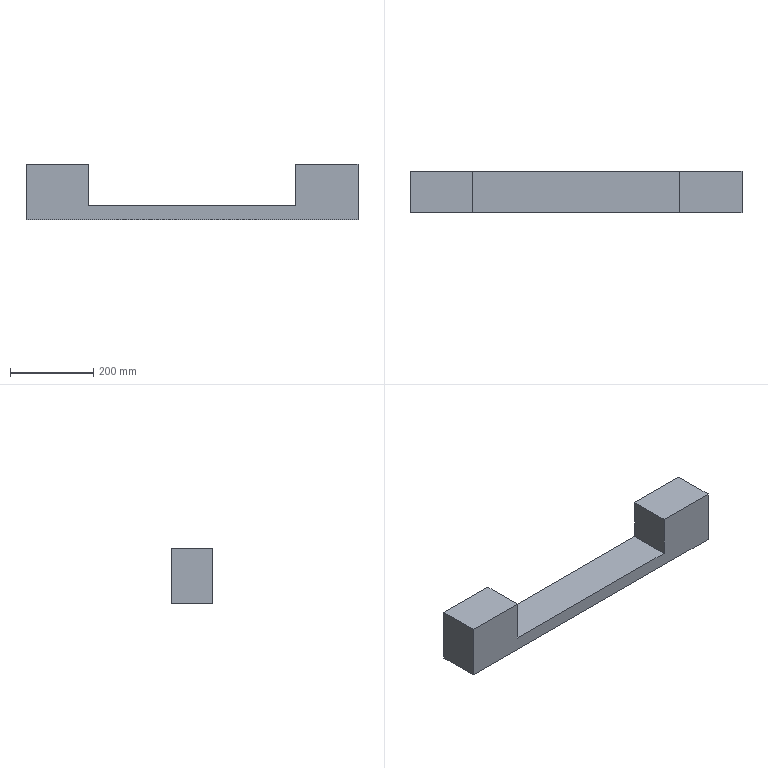Part | SolidWorks | features Split 3, Cut 2, Extrusion 1, MirrorPattern 1 | 1 solid | 20 faces | box 800 x 100 x 134 mm | volume 4312000 mm3 | plane 20
STEP:
#1=CARTESIAN_POINT('',(250.,100.,-33.));
#2=VERTEX_POINT('',#1);
#3=CARTESIAN_POINT('',(-250.,100.,-33.));
#4=VERTEX_POINT('',#3);
#5=CARTESIAN_POINT('',(-250.,100.,-33.));
#6=DIRECTION('',(-1.,0.,0.));
#7=VECTOR('',#6,1000.);
#8=LINE('',#5,#7);
#9=EDGE_CURVE('',#2,#4,#8,.T.);
#10=ORIENTED_EDGE('',*,*,#9,.F.);
#11=CARTESIAN_POINT('',(250.,100.,67.));
#12=VERTEX_POINT('',#11);
#13=CARTESIAN_POINT('',(250.,100.,167.));
#14=DIRECTION('',(0.,0.,-1.));
#15=VECTOR('',#14,1000.);
#16=LINE('',#13,#15);
#17=EDGE_CURVE('',#12,#2,#16,.T.);
#18=ORIENTED_EDGE('',*,*,#17,.F.);
#19=CARTESIAN_POINT('',(400.,100.,67.));
#20=VERTEX_POINT('',#19);
#21=CARTESIAN_POINT('',(-400.,100.,67.));
#22=DIRECTION('',(1.,0.,0.));
#23=VECTOR('',#22,1000.);
#24=LINE('',#21,#23);
#25=EDGE_CURVE('',#12,#20,#24,.T.);
#26=ORIENTED_EDGE('',*,*,#25,.T.);
#27=CARTESIAN_POINT('',(400.,100.,-67.));
#28=VERTEX_POINT('',#27);
#29=CARTESIAN_POINT('',(400.,100.,67.));
#30=DIRECTION('',(0.,0.,-1.));
#31=VECTOR('',#30,1000.);
#32=LINE('',#29,#31);
#33=EDGE_CURVE('',#20,#28,#32,.T.);
#34=ORIENTED_EDGE('',*,*,#33,.T.);
#35=CARTESIAN_POINT('',(-400.,100.,-67.));
#36=VERTEX_POINT('',#35);
#37=CARTESIAN_POINT('',(-400.,100.,-67.));
#38=DIRECTION('',(-1.,0.,0.));
#39=VECTOR('',#38,1000.);
#40=LINE('',#37,#39);
#41=EDGE_CURVE('',#28,#36,#40,.T.);
#42=ORIENTED_EDGE('',*,*,#41,.T.);
#43=CARTESIAN_POINT('',(-400.,100.,67.));
#44=VERTEX_POINT('',#43);
#45=CARTESIAN_POINT('',(-400.,100.,67.));
#46=DIRECTION('',(0.,0.,1.));
#47=VECTOR('',#46,1000.);
#48=LINE('',#45,#47);
#49=EDGE_CURVE('',#36,#44,#48,.T.);
#50=ORIENTED_EDGE('',*,*,#49,.T.);
#51=CARTESIAN_POINT('',(-250.,100.,67.));
#52=VERTEX_POINT('',#51);
#53=CARTESIAN_POINT('',(-400.,100.,67.));
#54=DIRECTION('',(1.,0.,0.));
#55=VECTOR('',#54,1000.);
#56=LINE('',#53,#55);
#57=EDGE_CURVE('',#44,#52,#56,.T.);
#58=ORIENTED_EDGE('',*,*,#57,.T.);
#59=CARTESIAN_POINT('',(-250.,100.,167.));
#60=DIRECTION('',(0.,0.,1.));
#61=VECTOR('',#60,1000.);
#62=LINE('',#59,#61);
#63=EDGE_CURVE('',#4,#52,#62,.T.);
#64=ORIENTED_EDGE('',*,*,#63,.F.);
#65=EDGE_LOOP('',(#10,#18,#26,#34,#42,#50,#58,#64));
#66=FACE_OUTER_BOUND('',#65,.T.);
#67=CARTESIAN_POINT('',(-380.,100.,47.));
#68=VERTEX_POINT('',#67);
#69=CARTESIAN_POINT('',(-270.,100.,47.));
#70=VERTEX_POINT('',#69);
#71=CARTESIAN_POINT('',(-380.,100.,47.));
#72=DIRECTION('',(1.,0.,0.));
#73=VECTOR('',#72,1000.);
#74=LINE('',#71,#73);
#75=EDGE_CURVE('',#68,#70,#74,.T.);
#76=ORIENTED_EDGE('',*,*,#75,.F.);
#77=CARTESIAN_POINT('',(-380.,100.,-33.));
#78=VERTEX_POINT('',#77);
#79=CARTESIAN_POINT('',(-380.,100.,47.));
#80=DIRECTION('',(0.,0.,1.));
#81=VECTOR('',#80,1000.);
#82=LINE('',#79,#81);
#83=EDGE_CURVE('',#78,#68,#82,.T.);
#84=ORIENTED_EDGE('',*,*,#83,.F.);
#85=CARTESIAN_POINT('',(-270.,100.,-33.));
#86=VERTEX_POINT('',#85);
#87=CARTESIAN_POINT('',(-380.,100.,-33.));
#88=DIRECTION('',(-1.,0.,0.));
#89=VECTOR('',#88,1000.);
#90=LINE('',#87,#89);
#91=EDGE_CURVE('',#86,#78,#90,.T.);
#92=ORIENTED_EDGE('',*,*,#91,.F.);
#93=CARTESIAN_POINT('',(-270.,100.,47.));
#94=DIRECTION('',(0.,0.,-1.));
#95=VECTOR('',#94,1000.);
#96=LINE('',#93,#95);
#97=EDGE_CURVE('',#70,#86,#96,.T.);
#98=ORIENTED_EDGE('',*,*,#97,.F.);
#99=EDGE_LOOP('',(#76,#84,#92,#98));
#100=FACE_BOUND('',#99,.T.);
#101=CARTESIAN_POINT('',(380.,100.,-33.));
#102=VERTEX_POINT('',#101);
#103=CARTESIAN_POINT('',(380.,100.,47.));
#104=VERTEX_POINT('',#103);
#105=CARTESIAN_POINT('',(380.,100.,47.));
#106=DIRECTION('',(0.,0.,1.));
#107=VECTOR('',#106,1000.);
#108=LINE('',#105,#107);
#109=EDGE_CURVE('',#102,#104,#108,.T.);
#110=ORIENTED_EDGE('',*,*,#109,.T.);
#111=CARTESIAN_POINT('',(270.,100.,47.));
#112=VERTEX_POINT('',#111);
#113=CARTESIAN_POINT('',(380.,100.,47.));
#114=DIRECTION('',(-1.,0.,0.));
#115=VECTOR('',#114,1000.);
#116=LINE('',#113,#115);
#117=EDGE_CURVE('',#104,#112,#116,.T.);
#118=ORIENTED_EDGE('',*,*,#117,.T.);
#119=CARTESIAN_POINT('',(270.,100.,-33.));
#120=VERTEX_POINT('',#119);
#121=CARTESIAN_POINT('',(270.,100.,47.));
#122=DIRECTION('',(0.,0.,-1.));
#123=VECTOR('',#122,1000.);
#124=LINE('',#121,#123);
#125=EDGE_CURVE('',#112,#120,#124,.T.);
#126=ORIENTED_EDGE('',*,*,#125,.T.);
#127=CARTESIAN_POINT('',(380.,100.,-33.));
#128=DIRECTION('',(1.,0.,0.));
#129=VECTOR('',#128,1000.);
#130=LINE('',#127,#129);
#131=EDGE_CURVE('',#120,#102,#130,.T.);
#132=ORIENTED_EDGE('',*,*,#131,.T.);
#133=EDGE_LOOP('',(#110,#118,#126,#132));
#134=FACE_BOUND('',#133,.T.);
#135=CARTESIAN_POINT('',(0.,100.,0.));
#136=DIRECTION('',(0.,-1.,0.));
#137=DIRECTION('',(0.,0.,-1.));
#138=AXIS2_PLACEMENT_3D('',#135,#136,#137);
#139=PLANE('',#138);
#140=ADVANCED_FACE('',(#66,#100,#134),#139,.F.);
#141=ORIENTED_EDGE('',*,*,#25,.F.);
#142=CARTESIAN_POINT('',(250.,0.,67.));
#143=VERTEX_POINT('',#142);
#144=CARTESIAN_POINT('',(250.,100.,67.));
#145=DIRECTION('',(0.,-1.,0.));
#146=VECTOR('',#145,1000.);
#147=LINE('',#144,#146);
#148=EDGE_CURVE('',#12,#143,#147,.T.);
#149=ORIENTED_EDGE('',*,*,#148,.T.);
#150=CARTESIAN_POINT('',(400.,0.,67.));
#151=VERTEX_POINT('',#150);
#152=CARTESIAN_POINT('',(-400.,0.,67.));
#153=DIRECTION('',(1.,0.,0.));
#154=VECTOR('',#153,1000.);
#155=LINE('',#152,#154);
#156=EDGE_CURVE('',#143,#151,#155,.T.);
#157=ORIENTED_EDGE('',*,*,#156,.T.);
#158=CARTESIAN_POINT('',(400.,100.,67.));
#159=DIRECTION('',(0.,-1.,0.));
#160=VECTOR('',#159,1000.);
#161=LINE('',#158,#160);
#162=EDGE_CURVE('',#20,#151,#161,.T.);
#163=ORIENTED_EDGE('',*,*,#162,.F.);
#164=EDGE_LOOP('',(#141,#149,#157,#163));
#165=FACE_OUTER_BOUND('',#164,.T.);
#166=CARTESIAN_POINT('',(-400.,100.,67.));
#167=DIRECTION('',(0.,0.,-1.));
#168=DIRECTION('',(-1.,0.,0.));
#169=AXIS2_PLACEMENT_3D('',#166,#167,#168);
#170=PLANE('',#169);
#171=ADVANCED_FACE('',(#165),#170,.F.);
#172=CARTESIAN_POINT('',(400.,0.,-67.));
#173=VERTEX_POINT('',#172);
#174=CARTESIAN_POINT('',(400.,0.,67.));
#175=DIRECTION('',(0.,0.,-1.));
#176=VECTOR('',#175,1000.);
#177=LINE('',#174,#176);
#178=EDGE_CURVE('',#151,#173,#177,.T.);
#179=ORIENTED_EDGE('',*,*,#178,.T.);
#180=CARTESIAN_POINT('',(400.,100.,-67.));
#181=DIRECTION('',(0.,-1.,0.));
#182=VECTOR('',#181,1000.);
#183=LINE('',#180,#182);
#184=EDGE_CURVE('',#28,#173,#183,.T.);
#185=ORIENTED_EDGE('',*,*,#184,.F.);
#186=ORIENTED_EDGE('',*,*,#33,.F.);
#187=ORIENTED_EDGE('',*,*,#162,.T.);
#188=EDGE_LOOP('',(#179,#185,#186,#187));
#189=FACE_OUTER_BOUND('',#188,.T.);
#190=CARTESIAN_POINT('',(400.,100.,67.));
#191=DIRECTION('',(-1.,0.,0.));
#192=DIRECTION('',(0.,0.,1.));
#193=AXIS2_PLACEMENT_3D('',#190,#191,#192);
#194=PLANE('',#193);
#195=ADVANCED_FACE('',(#189),#194,.F.);
#196=CARTESIAN_POINT('',(-400.,0.,-67.));
#197=VERTEX_POINT('',#196);
#198=CARTESIAN_POINT('',(-400.,0.,-67.));
#199=DIRECTION('',(-1.,0.,0.));
#200=VECTOR('',#199,1000.);
#201=LINE('',#198,#200);
#202=EDGE_CURVE('',#173,#197,#201,.T.);
#203=ORIENTED_EDGE('',*,*,#202,.T.);
#204=CARTESIAN_POINT('',(-400.,100.,-67.));
#205=DIRECTION('',(0.,-1.,0.));
#206=VECTOR('',#205,1000.);
#207=LINE('',#204,#206);
#208=EDGE_CURVE('',#36,#197,#207,.T.);
#209=ORIENTED_EDGE('',*,*,#208,.F.);
#210=ORIENTED_EDGE('',*,*,#41,.F.);
#211=ORIENTED_EDGE('',*,*,#184,.T.);
#212=EDGE_LOOP('',(#203,#209,#210,#211));
#213=FACE_OUTER_BOUND('',#212,.T.);
#214=CARTESIAN_POINT('',(-400.,100.,-67.));
#215=DIRECTION('',(0.,0.,1.));
#216=DIRECTION('',(1.,0.,0.));
#217=AXIS2_PLACEMENT_3D('',#214,#215,#216);
#218=PLANE('',#217);
#219=ADVANCED_FACE('',(#213),#218,.F.);
#220=CARTESIAN_POINT('',(-400.,0.,67.));
#221=VERTEX_POINT('',#220);
#222=CARTESIAN_POINT('',(-400.,0.,67.));
#223=DIRECTION('',(0.,0.,1.));
#224=VECTOR('',#223,1000.);
#225=LINE('',#222,#224);
#226=EDGE_CURVE('',#197,#221,#225,.T.);
#227=ORIENTED_EDGE('',*,*,#226,.T.);
#228=CARTESIAN_POINT('',(-400.,100.,67.));
#229=DIRECTION('',(0.,-1.,0.));
#230=VECTOR('',#229,1000.);
#231=LINE('',#228,#230);
#232=EDGE_CURVE('',#44,#221,#231,.T.);
#233=ORIENTED_EDGE('',*,*,#232,.F.);
#234=ORIENTED_EDGE('',*,*,#49,.F.);
#235=ORIENTED_EDGE('',*,*,#208,.T.);
#236=EDGE_LOOP('',(#227,#233,#234,#235));
#237=FACE_OUTER_BOUND('',#236,.T.);
#238=CARTESIAN_POINT('',(-400.,100.,67.));
#239=DIRECTION('',(1.,0.,0.));
#240=DIRECTION('',(0.,0.,-1.));
#241=AXIS2_PLACEMENT_3D('',#238,#239,#240);
#242=PLANE('',#241);
#243=ADVANCED_FACE('',(#237),#242,.F.);
#244=CARTESIAN_POINT('',(-250.,0.,67.));
#245=VERTEX_POINT('',#244);
#246=CARTESIAN_POINT('',(-400.,0.,67.));
#247=DIRECTION('',(1.,0.,0.));
#248=VECTOR('',#247,1000.);
#249=LINE('',#246,#248);
#250=EDGE_CURVE('',#221,#245,#249,.T.);
#251=ORIENTED_EDGE('',*,*,#250,.T.);
#252=CARTESIAN_POINT('',(-250.,100.,67.));
#253=DIRECTION('',(0.,1.,0.));
#254=VECTOR('',#253,1000.);
#255=LINE('',#252,#254);
#256=EDGE_CURVE('',#245,#52,#255,.T.);
#257=ORIENTED_EDGE('',*,*,#256,.T.);
#258=ORIENTED_EDGE('',*,*,#57,.F.);
#259=ORIENTED_EDGE('',*,*,#232,.T.);
#260=EDGE_LOOP('',(#251,#257,#258,#259));
#261=FACE_OUTER_BOUND('',#260,.T.);
#262=CARTESIAN_POINT('',(-400.,100.,67.));
#263=DIRECTION('',(0.,0.,-1.));
#264=DIRECTION('',(-1.,0.,0.));
#265=AXIS2_PLACEMENT_3D('',#262,#263,#264);
#266=PLANE('',#265);
#267=ADVANCED_FACE('',(#261),#266,.F.);
#268=CARTESIAN_POINT('',(250.,0.,-33.));
#269=VERTEX_POINT('',#268);
#270=CARTESIAN_POINT('',(250.,0.,0.));
#271=DIRECTION('',(0.,0.,1.));
#272=VECTOR('',#271,1000.);
#273=LINE('',#270,#272);
#274=EDGE_CURVE('',#269,#143,#273,.T.);
#275=ORIENTED_EDGE('',*,*,#274,.F.);
#276=CARTESIAN_POINT('',(-250.,0.,-33.));
#277=VERTEX_POINT('',#276);
#278=CARTESIAN_POINT('',(-250.,0.,-33.));
#279=DIRECTION('',(-1.,0.,0.));
#280=VECTOR('',#279,1000.);
#281=LINE('',#278,#280);
#282=EDGE_CURVE('',#269,#277,#281,.T.);
#283=ORIENTED_EDGE('',*,*,#282,.T.);
#284=CARTESIAN_POINT('',(-250.,0.,167.));
#285=DIRECTION('',(0.,0.,1.));
#286=VECTOR('',#285,1000.);
#287=LINE('',#284,#286);
#288=EDGE_CURVE('',#277,#245,#287,.T.);
#289=ORIENTED_EDGE('',*,*,#288,.T.);
#290=ORIENTED_EDGE('',*,*,#250,.F.);
#291=ORIENTED_EDGE('',*,*,#226,.F.);
#292=ORIENTED_EDGE('',*,*,#202,.F.);
#293=ORIENTED_EDGE('',*,*,#178,.F.);
#294=ORIENTED_EDGE('',*,*,#156,.F.);
#295=EDGE_LOOP('',(#275,#283,#289,#290,#291,#292,#293,#294));
#296=FACE_OUTER_BOUND('',#295,.T.);
#297=CARTESIAN_POINT('',(0.,0.,0.));
#298=DIRECTION('',(0.,-1.,0.));
#299=DIRECTION('',(0.,0.,-1.));
#300=AXIS2_PLACEMENT_3D('',#297,#298,#299);
#301=PLANE('',#300);
#302=ADVANCED_FACE('',(#296),#301,.T.);
#303=ORIENTED_EDGE('',*,*,#17,.T.);
#304=CARTESIAN_POINT('',(250.,0.,-33.));
#305=DIRECTION('',(0.,1.,0.));
#306=VECTOR('',#305,1000.);
#307=LINE('',#304,#306);
#308=EDGE_CURVE('',#269,#2,#307,.T.);
#309=ORIENTED_EDGE('',*,*,#308,.F.);
#310=ORIENTED_EDGE('',*,*,#274,.T.);
#311=ORIENTED_EDGE('',*,*,#148,.F.);
#312=EDGE_LOOP('',(#303,#309,#310,#311));
#313=FACE_OUTER_BOUND('',#312,.T.);
#314=CARTESIAN_POINT('',(250.,0.,167.));
#315=DIRECTION('',(1.,0.,0.));
#316=DIRECTION('',(0.,0.,-1.));
#317=AXIS2_PLACEMENT_3D('',#314,#315,#316);
#318=PLANE('',#317);
#319=ADVANCED_FACE('',(#313),#318,.F.);
#320=ORIENTED_EDGE('',*,*,#288,.F.);
#321=CARTESIAN_POINT('',(-250.,0.,-33.));
#322=DIRECTION('',(0.,1.,0.));
#323=VECTOR('',#322,1000.);
#324=LINE('',#321,#323);
#325=EDGE_CURVE('',#277,#4,#324,.T.);
#326=ORIENTED_EDGE('',*,*,#325,.T.);
#327=ORIENTED_EDGE('',*,*,#63,.T.);
#328=ORIENTED_EDGE('',*,*,#256,.F.);
#329=EDGE_LOOP('',(#320,#326,#327,#328));
#330=FACE_OUTER_BOUND('',#329,.T.);
#331=CARTESIAN_POINT('',(-250.,0.,167.));
#332=DIRECTION('',(-1.,0.,0.));
#333=DIRECTION('',(0.,0.,1.));
#334=AXIS2_PLACEMENT_3D('',#331,#332,#333);
#335=PLANE('',#334);
#336=ADVANCED_FACE('',(#330),#335,.F.);
#337=ORIENTED_EDGE('',*,*,#9,.T.);
#338=ORIENTED_EDGE('',*,*,#325,.F.);
#339=ORIENTED_EDGE('',*,*,#282,.F.);
#340=ORIENTED_EDGE('',*,*,#308,.T.);
#341=EDGE_LOOP('',(#337,#338,#339,#340));
#342=FACE_OUTER_BOUND('',#341,.T.);
#343=CARTESIAN_POINT('',(-250.,0.,-33.));
#344=DIRECTION('',(0.,0.,-1.));
#345=DIRECTION('',(-1.,0.,0.));
#346=AXIS2_PLACEMENT_3D('',#343,#344,#345);
#347=PLANE('',#346);
#348=ADVANCED_FACE('',(#342),#347,.F.);
#349=ORIENTED_EDGE('',*,*,#83,.T.);
#350=CARTESIAN_POINT('',(-380.,20.,47.));
#351=VERTEX_POINT('',#350);
#352=CARTESIAN_POINT('',(-380.,20.,47.));
#353=DIRECTION('',(0.,1.,0.));
#354=VECTOR('',#353,1000.);
#355=LINE('',#352,#354);
#356=EDGE_CURVE('',#351,#68,#355,.T.);
#357=ORIENTED_EDGE('',*,*,#356,.F.);
#358=CARTESIAN_POINT('',(-380.,20.,-33.));
#359=VERTEX_POINT('',#358);
#360=CARTESIAN_POINT('',(-380.,20.,47.));
#361=DIRECTION('',(0.,0.,1.));
#362=VECTOR('',#361,1000.);
#363=LINE('',#360,#362);
#364=EDGE_CURVE('',#359,#351,#363,.T.);
#365=ORIENTED_EDGE('',*,*,#364,.F.);
#366=CARTESIAN_POINT('',(-380.,20.,-33.));
#367=DIRECTION('',(0.,1.,0.));
#368=VECTOR('',#367,1000.);
#369=LINE('',#366,#368);
#370=EDGE_CURVE('',#359,#78,#369,.T.);
#371=ORIENTED_EDGE('',*,*,#370,.T.);
#372=EDGE_LOOP('',(#349,#357,#365,#371));
#373=FACE_OUTER_BOUND('',#372,.T.);
#374=CARTESIAN_POINT('',(-380.,20.,47.));
#375=DIRECTION('',(-1.,0.,0.));
#376=DIRECTION('',(0.,0.,1.));
#377=AXIS2_PLACEMENT_3D('',#374,#375,#376);
#378=PLANE('',#377);
#379=ADVANCED_FACE('',(#373),#378,.F.);
#380=ORIENTED_EDGE('',*,*,#91,.T.);
#381=ORIENTED_EDGE('',*,*,#370,.F.);
#382=CARTESIAN_POINT('',(-270.,20.,-33.));
#383=VERTEX_POINT('',#382);
#384=CARTESIAN_POINT('',(-380.,20.,-33.));
#385=DIRECTION('',(-1.,0.,0.));
#386=VECTOR('',#385,1000.);
#387=LINE('',#384,#386);
#388=EDGE_CURVE('',#383,#359,#387,.T.);
#389=ORIENTED_EDGE('',*,*,#388,.F.);
#390=CARTESIAN_POINT('',(-270.,20.,-33.));
#391=DIRECTION('',(0.,1.,0.));
#392=VECTOR('',#391,1000.);
#393=LINE('',#390,#392);
#394=EDGE_CURVE('',#383,#86,#393,.T.);
#395=ORIENTED_EDGE('',*,*,#394,.T.);
#396=EDGE_LOOP('',(#380,#381,#389,#395));
#397=FACE_OUTER_BOUND('',#396,.T.);
#398=CARTESIAN_POINT('',(-380.,20.,-33.));
#399=DIRECTION('',(0.,0.,-1.));
#400=DIRECTION('',(-1.,0.,0.));
#401=AXIS2_PLACEMENT_3D('',#398,#399,#400);
#402=PLANE('',#401);
#403=ADVANCED_FACE('',(#397),#402,.F.);
#404=ORIENTED_EDGE('',*,*,#97,.T.);
#405=ORIENTED_EDGE('',*,*,#394,.F.);
#406=CARTESIAN_POINT('',(-270.,20.,47.));
#407=VERTEX_POINT('',#406);
#408=CARTESIAN_POINT('',(-270.,20.,47.));
#409=DIRECTION('',(0.,0.,-1.));
#410=VECTOR('',#409,1000.);
#411=LINE('',#408,#410);
#412=EDGE_CURVE('',#407,#383,#411,.T.);
#413=ORIENTED_EDGE('',*,*,#412,.F.);
#414=CARTESIAN_POINT('',(-270.,20.,47.));
#415=DIRECTION('',(0.,1.,0.));
#416=VECTOR('',#415,1000.);
#417=LINE('',#414,#416);
#418=EDGE_CURVE('',#407,#70,#417,.T.);
#419=ORIENTED_EDGE('',*,*,#418,.T.);
#420=EDGE_LOOP('',(#404,#405,#413,#419));
#421=FACE_OUTER_BOUND('',#420,.T.);
#422=CARTESIAN_POINT('',(-270.,20.,47.));
#423=DIRECTION('',(1.,0.,0.));
#424=DIRECTION('',(0.,0.,-1.));
#425=AXIS2_PLACEMENT_3D('',#422,#423,#424);
#426=PLANE('',#425);
#427=ADVANCED_FACE('',(#421),#426,.F.);
#428=ORIENTED_EDGE('',*,*,#75,.T.);
#429=ORIENTED_EDGE('',*,*,#418,.F.);
#430=CARTESIAN_POINT('',(-380.,20.,47.));
#431=DIRECTION('',(1.,0.,0.));
#432=VECTOR('',#431,1000.);
#433=LINE('',#430,#432);
#434=EDGE_CURVE('',#351,#407,#433,.T.);
#435=ORIENTED_EDGE('',*,*,#434,.F.);
#436=ORIENTED_EDGE('',*,*,#356,.T.);
#437=EDGE_LOOP('',(#428,#429,#435,#436));
#438=FACE_OUTER_BOUND('',#437,.T.);
#439=CARTESIAN_POINT('',(-380.,20.,47.));
#440=DIRECTION('',(0.,0.,1.));
#441=DIRECTION('',(1.,0.,0.));
#442=AXIS2_PLACEMENT_3D('',#439,#440,#441);
#443=PLANE('',#442);
#444=ADVANCED_FACE('',(#438),#443,.F.);
#445=ORIENTED_EDGE('',*,*,#364,.T.);
#446=ORIENTED_EDGE('',*,*,#434,.T.);
#447=ORIENTED_EDGE('',*,*,#412,.T.);
#448=ORIENTED_EDGE('',*,*,#388,.T.);
#449=EDGE_LOOP('',(#445,#446,#447,#448));
#450=FACE_OUTER_BOUND('',#449,.T.);
#451=CARTESIAN_POINT('',(0.,20.,0.));
#452=DIRECTION('',(0.,-1.,0.));
#453=DIRECTION('',(0.,0.,-1.));
#454=AXIS2_PLACEMENT_3D('',#451,#452,#453);
#455=PLANE('',#454);
#456=ADVANCED_FACE('',(#450),#455,.F.);
#457=ORIENTED_EDGE('',*,*,#109,.F.);
#458=CARTESIAN_POINT('',(380.,20.,-33.));
#459=VERTEX_POINT('',#458);
#460=CARTESIAN_POINT('',(380.,20.,-33.));
#461=DIRECTION('',(0.,1.,0.));
#462=VECTOR('',#461,1000.);
#463=LINE('',#460,#462);
#464=EDGE_CURVE('',#459,#102,#463,.T.);
#465=ORIENTED_EDGE('',*,*,#464,.F.);
#466=CARTESIAN_POINT('',(380.,20.,47.));
#467=VERTEX_POINT('',#466);
#468=CARTESIAN_POINT('',(380.,20.,47.));
#469=DIRECTION('',(0.,0.,1.));
#470=VECTOR('',#469,1000.);
#471=LINE('',#468,#470);
#472=EDGE_CURVE('',#459,#467,#471,.T.);
#473=ORIENTED_EDGE('',*,*,#472,.T.);
#474=CARTESIAN_POINT('',(380.,20.,47.));
#475=DIRECTION('',(0.,1.,0.));
#476=VECTOR('',#475,1000.);
#477=LINE('',#474,#476);
#478=EDGE_CURVE('',#467,#104,#477,.T.);
#479=ORIENTED_EDGE('',*,*,#478,.T.);
#480=EDGE_LOOP('',(#457,#465,#473,#479));
#481=FACE_OUTER_BOUND('',#480,.T.);
#482=CARTESIAN_POINT('',(380.,20.,47.));
#483=DIRECTION('',(-1.,0.,0.));
#484=DIRECTION('',(0.,0.,1.));
#485=AXIS2_PLACEMENT_3D('',#482,#483,#484);
#486=PLANE('',#485);
#487=ADVANCED_FACE('',(#481),#486,.T.);
#488=ORIENTED_EDGE('',*,*,#117,.F.);
#489=ORIENTED_EDGE('',*,*,#478,.F.);
#490=CARTESIAN_POINT('',(270.,20.,47.));
#491=VERTEX_POINT('',#490);
#492=CARTESIAN_POINT('',(380.,20.,47.));
#493=DIRECTION('',(-1.,0.,0.));
#494=VECTOR('',#493,1000.);
#495=LINE('',#492,#494);
#496=EDGE_CURVE('',#467,#491,#495,.T.);
#497=ORIENTED_EDGE('',*,*,#496,.T.);
#498=CARTESIAN_POINT('',(270.,20.,47.));
#499=DIRECTION('',(0.,1.,0.));
#500=VECTOR('',#499,1000.);
#501=LINE('',#498,#500);
#502=EDGE_CURVE('',#491,#112,#501,.T.);
#503=ORIENTED_EDGE('',*,*,#502,.T.);
#504=EDGE_LOOP('',(#488,#489,#497,#503));
#505=FACE_OUTER_BOUND('',#504,.T.);
#506=CARTESIAN_POINT('',(380.,20.,47.));
#507=DIRECTION('',(0.,0.,-1.));
#508=DIRECTION('',(-1.,0.,0.));
#509=AXIS2_PLACEMENT_3D('',#506,#507,#508);
#510=PLANE('',#509);
#511=ADVANCED_FACE('',(#505),#510,.T.);
#512=ORIENTED_EDGE('',*,*,#125,.F.);
#513=ORIENTED_EDGE('',*,*,#502,.F.);
#514=CARTESIAN_POINT('',(270.,20.,-33.));
#515=VERTEX_POINT('',#514);
#516=CARTESIAN_POINT('',(270.,20.,47.));
#517=DIRECTION('',(0.,0.,-1.));
#518=VECTOR('',#517,1000.);
#519=LINE('',#516,#518);
#520=EDGE_CURVE('',#491,#515,#519,.T.);
#521=ORIENTED_EDGE('',*,*,#520,.T.);
#522=CARTESIAN_POINT('',(270.,20.,-33.));
#523=DIRECTION('',(0.,1.,0.));
#524=VECTOR('',#523,1000.);
#525=LINE('',#522,#524);
#526=EDGE_CURVE('',#515,#120,#525,.T.);
#527=ORIENTED_EDGE('',*,*,#526,.T.);
#528=EDGE_LOOP('',(#512,#513,#521,#527));
#529=FACE_OUTER_BOUND('',#528,.T.);
#530=CARTESIAN_POINT('',(270.,20.,47.));
#531=DIRECTION('',(1.,0.,0.));
#532=DIRECTION('',(0.,0.,-1.));
#533=AXIS2_PLACEMENT_3D('',#530,#531,#532);
#534=PLANE('',#533);
#535=ADVANCED_FACE('',(#529),#534,.T.);
#536=ORIENTED_EDGE('',*,*,#131,.F.);
#537=ORIENTED_EDGE('',*,*,#526,.F.);
#538=CARTESIAN_POINT('',(380.,20.,-33.));
#539=DIRECTION('',(1.,0.,0.));
#540=VECTOR('',#539,1000.);
#541=LINE('',#538,#540);
#542=EDGE_CURVE('',#515,#459,#541,.T.);
#543=ORIENTED_EDGE('',*,*,#542,.T.);
#544=ORIENTED_EDGE('',*,*,#464,.T.);
#545=EDGE_LOOP('',(#536,#537,#543,#544));
#546=FACE_OUTER_BOUND('',#545,.T.);
#547=CARTESIAN_POINT('',(380.,20.,-33.));
#548=DIRECTION('',(0.,0.,1.));
#549=DIRECTION('',(1.,0.,0.));
#550=AXIS2_PLACEMENT_3D('',#547,#548,#549);
#551=PLANE('',#550);
#552=ADVANCED_FACE('',(#546),#551,.T.);
#553=ORIENTED_EDGE('',*,*,#472,.F.);
#554=ORIENTED_EDGE('',*,*,#542,.F.);
#555=ORIENTED_EDGE('',*,*,#520,.F.);
#556=ORIENTED_EDGE('',*,*,#496,.F.);
#557=EDGE_LOOP('',(#553,#554,#555,#556));
#558=FACE_OUTER_BOUND('',#557,.T.);
#559=CARTESIAN_POINT('',(0.,20.,0.));
#560=DIRECTION('',(0.,-1.,0.));
#561=DIRECTION('',(0.,0.,-1.));
#562=AXIS2_PLACEMENT_3D('',#559,#560,#561);
#563=PLANE('',#562);
#564=ADVANCED_FACE('',(#558),#563,.F.);
#565=CLOSED_SHELL('',(#140,#171,#195,#219,#243,#267,#302,#319,#336,#348,#379,#403,#427,#444,#456,#487,#511,#535,#552,#564));
#566=MANIFOLD_SOLID_BREP('',#565);
#567=CARTESIAN_POINT('',(0.,0.,0.));
#568=DIRECTION('',(0.,0.,1.));
#569=DIRECTION('',(1.,0.,0.));
#570=AXIS2_PLACEMENT_3D('',#567,#568,#569);
#571=(LENGTH_UNIT()NAMED_UNIT(*)SI_UNIT(.MILLI.,.METRE.));
#572=UNCERTAINTY_MEASURE_WITH_UNIT(LENGTH_MEASURE(0.00001),#571,'','');
#573=(NAMED_UNIT(*)PLANE_ANGLE_UNIT()SI_UNIT($,.RADIAN.));
#574=(NAMED_UNIT(*)SI_UNIT($,.STERADIAN.)SOLID_ANGLE_UNIT());
#575=(GEOMETRIC_REPRESENTATION_CONTEXT(3)GLOBAL_UNCERTAINTY_ASSIGNED_CONTEXT((#572))GLOBAL_UNIT_ASSIGNED_CONTEXT((#571,#573,#574))REPRESENTATION_CONTEXT('',''));
#576=ADVANCED_BREP_SHAPE_REPRESENTATION('',(#566,#570),#575);